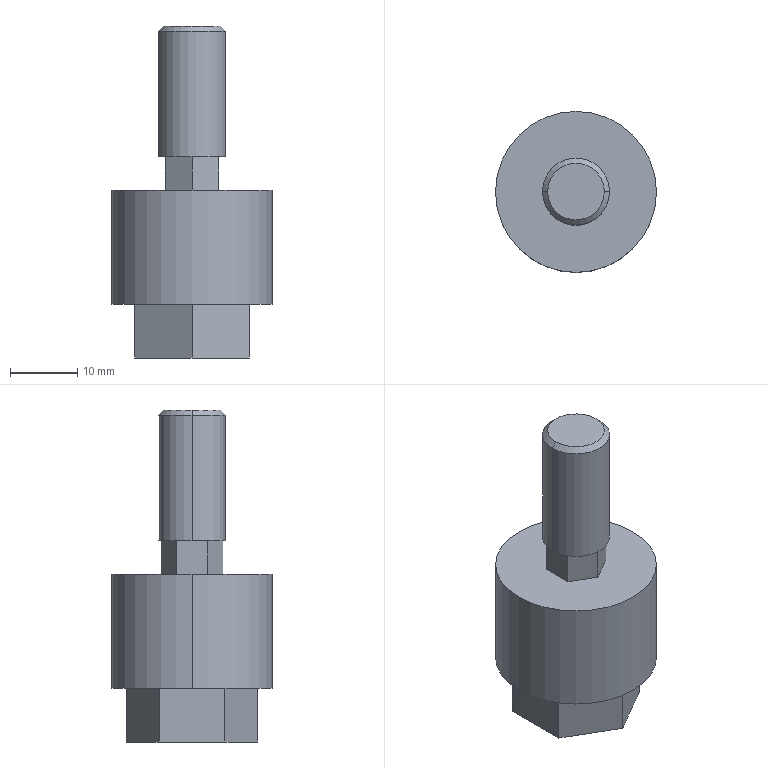Part | STEP file | JA30_10_125_JA30-10-125 | 1 solid | 28 faces | box 24 x 24 x 49.5 mm | volume 10958 mm3 | plane 18 | cylinder 6 | cone 4 | commonest cylinder face diameters 8.647 x2 10 x2 24 x2
STEP:
#1=CARTESIAN_POINT('',(-5.,0.,48.733));
#2=VERTEX_POINT('',#1);
#3=CARTESIAN_POINT('',(5.,0.,48.733));
#4=VERTEX_POINT('',#3);
#5=CARTESIAN_POINT('',(0.,0.,48.733));
#6=DIRECTION('',(0.,0.,-1.));
#7=DIRECTION('',(-1.,0.,0.));
#8=AXIS2_PLACEMENT_3D('',#5,#6,#7);
#9=CIRCLE('',#8,5.);
#10=EDGE_CURVE('',#2,#4,#9,.T.);
#11=ORIENTED_EDGE('',*,*,#10,.T.);
#12=CARTESIAN_POINT('',(5.,0.,30.));
#13=VERTEX_POINT('',#12);
#14=CARTESIAN_POINT('',(5.,0.,30.));
#15=DIRECTION('',(0.,0.,-1.));
#16=VECTOR('',#15,1000.);
#17=LINE('',#14,#16);
#18=EDGE_CURVE('',#4,#13,#17,.T.);
#19=ORIENTED_EDGE('',*,*,#18,.T.);
#20=CARTESIAN_POINT('',(-5.,0.,30.));
#21=VERTEX_POINT('',#20);
#22=CARTESIAN_POINT('',(0.,0.,30.));
#23=DIRECTION('',(0.,0.,-1.));
#24=DIRECTION('',(-1.,0.,0.));
#25=AXIS2_PLACEMENT_3D('',#22,#23,#24);
#26=CIRCLE('',#25,5.);
#27=EDGE_CURVE('',#21,#13,#26,.T.);
#28=ORIENTED_EDGE('',*,*,#27,.F.);
#29=CARTESIAN_POINT('',(-5.,0.,30.));
#30=DIRECTION('',(0.,0.,-1.));
#31=VECTOR('',#30,1000.);
#32=LINE('',#29,#31);
#33=EDGE_CURVE('',#2,#21,#32,.T.);
#34=ORIENTED_EDGE('',*,*,#33,.F.);
#35=EDGE_LOOP('',(#11,#19,#28,#34));
#36=FACE_OUTER_BOUND('',#35,.T.);
#37=CARTESIAN_POINT('',(0.,0.,30.));
#38=DIRECTION('',(0.,0.,-1.));
#39=DIRECTION('',(-1.,0.,0.));
#40=AXIS2_PLACEMENT_3D('',#37,#38,#39);
#41=CYLINDRICAL_SURFACE('',#40,5.);
#42=ADVANCED_FACE('',(#36),#41,.T.);
#43=CARTESIAN_POINT('',(-4.233,0.,49.5));
#44=VERTEX_POINT('',#43);
#45=CARTESIAN_POINT('',(4.233,0.,49.5));
#46=VERTEX_POINT('',#45);
#47=CARTESIAN_POINT('',(0.,0.,49.5));
#48=DIRECTION('',(0.,0.,-1.));
#49=DIRECTION('',(-1.,0.,0.));
#50=AXIS2_PLACEMENT_3D('',#47,#48,#49);
#51=CIRCLE('',#50,4.233);
#52=EDGE_CURVE('',#44,#46,#51,.T.);
#53=ORIENTED_EDGE('',*,*,#52,.T.);
#54=CARTESIAN_POINT('',(5.,0.,48.733));
#55=DIRECTION('',(0.7071,0.,-0.7071));
#56=VECTOR('',#55,1000.);
#57=LINE('',#54,#56);
#58=EDGE_CURVE('',#46,#4,#57,.T.);
#59=ORIENTED_EDGE('',*,*,#58,.T.);
#60=ORIENTED_EDGE('',*,*,#10,.F.);
#61=CARTESIAN_POINT('',(-5.,0.,48.733));
#62=DIRECTION('',(-0.7071,0.,-0.7071));
#63=VECTOR('',#62,1000.);
#64=LINE('',#61,#63);
#65=EDGE_CURVE('',#44,#2,#64,.T.);
#66=ORIENTED_EDGE('',*,*,#65,.F.);
#67=EDGE_LOOP('',(#53,#59,#60,#66));
#68=FACE_OUTER_BOUND('',#67,.T.);
#69=CARTESIAN_POINT('',(0.,0.,48.733));
#70=DIRECTION('',(0.,0.,-1.));
#71=DIRECTION('',(-1.,0.,0.));
#72=AXIS2_PLACEMENT_3D('',#69,#70,#71);
#73=CONICAL_SURFACE('',#72,5.,0.7854);
#74=ADVANCED_FACE('',(#68),#73,.T.);
#75=CARTESIAN_POINT('',(4.324,0.,0.6765));
#76=VERTEX_POINT('',#75);
#77=CARTESIAN_POINT('',(-4.324,0.,0.6765));
#78=VERTEX_POINT('',#77);
#79=CARTESIAN_POINT('',(0.,0.,0.6765));
#80=DIRECTION('',(0.,0.,-1.));
#81=DIRECTION('',(-1.,0.,0.));
#82=AXIS2_PLACEMENT_3D('',#79,#80,#81);
#83=CIRCLE('',#82,4.324);
#84=EDGE_CURVE('',#76,#78,#83,.T.);
#85=ORIENTED_EDGE('',*,*,#84,.F.);
#86=CARTESIAN_POINT('',(5.,0.,0.));
#87=VERTEX_POINT('',#86);
#88=CARTESIAN_POINT('',(4.324,0.,0.6765));
#89=DIRECTION('',(0.7071,0.,-0.7071));
#90=VECTOR('',#89,1000.);
#91=LINE('',#88,#90);
#92=EDGE_CURVE('',#76,#87,#91,.T.);
#93=ORIENTED_EDGE('',*,*,#92,.T.);
#94=CARTESIAN_POINT('',(-5.,0.,0.));
#95=VERTEX_POINT('',#94);
#96=CARTESIAN_POINT('',(0.,0.,0.));
#97=DIRECTION('',(0.,0.,-1.));
#98=DIRECTION('',(-1.,0.,0.));
#99=AXIS2_PLACEMENT_3D('',#96,#97,#98);
#100=CIRCLE('',#99,5.);
#101=EDGE_CURVE('',#87,#95,#100,.T.);
#102=ORIENTED_EDGE('',*,*,#101,.T.);
#103=CARTESIAN_POINT('',(-4.324,0.,0.6765));
#104=DIRECTION('',(-0.7071,0.,-0.7071));
#105=VECTOR('',#104,1000.);
#106=LINE('',#103,#105);
#107=EDGE_CURVE('',#78,#95,#106,.T.);
#108=ORIENTED_EDGE('',*,*,#107,.F.);
#109=EDGE_LOOP('',(#85,#93,#102,#108));
#110=FACE_OUTER_BOUND('',#109,.T.);
#111=CARTESIAN_POINT('',(0.,0.,0.6765));
#112=DIRECTION('',(0.,0.,-1.));
#113=DIRECTION('',(-1.,0.,0.));
#114=AXIS2_PLACEMENT_3D('',#111,#112,#113);
#115=CONICAL_SURFACE('',#114,4.324,0.7854);
#116=ADVANCED_FACE('',(#110),#115,.F.);
#117=CARTESIAN_POINT('',(4.324,0.,9.));
#118=VERTEX_POINT('',#117);
#119=CARTESIAN_POINT('',(-4.324,0.,9.));
#120=VERTEX_POINT('',#119);
#121=CARTESIAN_POINT('',(0.,0.,9.));
#122=DIRECTION('',(0.,0.,-1.));
#123=DIRECTION('',(-1.,0.,0.));
#124=AXIS2_PLACEMENT_3D('',#121,#122,#123);
#125=CIRCLE('',#124,4.324);
#126=EDGE_CURVE('',#118,#120,#125,.T.);
#127=ORIENTED_EDGE('',*,*,#126,.F.);
#128=CARTESIAN_POINT('',(4.324,0.,0.));
#129=DIRECTION('',(0.,0.,-1.));
#130=VECTOR('',#129,1000.);
#131=LINE('',#128,#130);
#132=EDGE_CURVE('',#118,#76,#131,.T.);
#133=ORIENTED_EDGE('',*,*,#132,.T.);
#134=ORIENTED_EDGE('',*,*,#84,.T.);
#135=CARTESIAN_POINT('',(-4.324,0.,0.));
#136=DIRECTION('',(0.,0.,-1.));
#137=VECTOR('',#136,1000.);
#138=LINE('',#135,#137);
#139=EDGE_CURVE('',#120,#78,#138,.T.);
#140=ORIENTED_EDGE('',*,*,#139,.F.);
#141=EDGE_LOOP('',(#127,#133,#134,#140));
#142=FACE_OUTER_BOUND('',#141,.T.);
#143=CARTESIAN_POINT('',(0.,0.,0.));
#144=DIRECTION('',(0.,0.,-1.));
#145=DIRECTION('',(-1.,0.,0.));
#146=AXIS2_PLACEMENT_3D('',#143,#144,#145);
#147=CYLINDRICAL_SURFACE('',#146,4.324);
#148=ADVANCED_FACE('',(#142),#147,.F.);
#149=CARTESIAN_POINT('',(-12.,0.,25.));
#150=VERTEX_POINT('',#149);
#151=CARTESIAN_POINT('',(12.,0.,25.));
#152=VERTEX_POINT('',#151);
#153=CARTESIAN_POINT('',(0.,0.,25.));
#154=DIRECTION('',(0.,0.,-1.));
#155=DIRECTION('',(-1.,0.,0.));
#156=AXIS2_PLACEMENT_3D('',#153,#154,#155);
#157=CIRCLE('',#156,12.);
#158=EDGE_CURVE('',#150,#152,#157,.T.);
#159=ORIENTED_EDGE('',*,*,#158,.T.);
#160=CARTESIAN_POINT('',(12.,0.,8.));
#161=VERTEX_POINT('',#160);
#162=CARTESIAN_POINT('',(12.,0.,0.));
#163=DIRECTION('',(0.,0.,-1.));
#164=VECTOR('',#163,1000.);
#165=LINE('',#162,#164);
#166=EDGE_CURVE('',#152,#161,#165,.T.);
#167=ORIENTED_EDGE('',*,*,#166,.T.);
#168=CARTESIAN_POINT('',(-12.,0.,8.));
#169=VERTEX_POINT('',#168);
#170=CARTESIAN_POINT('',(0.,0.,8.));
#171=DIRECTION('',(0.,0.,-1.));
#172=DIRECTION('',(-1.,0.,0.));
#173=AXIS2_PLACEMENT_3D('',#170,#171,#172);
#174=CIRCLE('',#173,12.);
#175=EDGE_CURVE('',#169,#161,#174,.T.);
#176=ORIENTED_EDGE('',*,*,#175,.F.);
#177=CARTESIAN_POINT('',(-12.,0.,0.));
#178=DIRECTION('',(0.,0.,-1.));
#179=VECTOR('',#178,1000.);
#180=LINE('',#177,#179);
#181=EDGE_CURVE('',#150,#169,#180,.T.);
#182=ORIENTED_EDGE('',*,*,#181,.F.);
#183=EDGE_LOOP('',(#159,#167,#176,#182));
#184=FACE_OUTER_BOUND('',#183,.T.);
#185=CARTESIAN_POINT('',(0.,0.,0.));
#186=DIRECTION('',(0.,0.,-1.));
#187=DIRECTION('',(-1.,0.,0.));
#188=AXIS2_PLACEMENT_3D('',#185,#186,#187);
#189=CYLINDRICAL_SURFACE('',#188,12.);
#190=ADVANCED_FACE('',(#184),#189,.T.);
#191=CARTESIAN_POINT('',(0.,4.619,30.));
#192=VERTEX_POINT('',#191);
#193=CARTESIAN_POINT('',(-4.,2.309,30.));
#194=VERTEX_POINT('',#193);
#195=CARTESIAN_POINT('',(0.,4.619,30.));
#196=DIRECTION('',(-0.866,-0.5,0.));
#197=VECTOR('',#196,1000.);
#198=LINE('',#195,#197);
#199=EDGE_CURVE('',#192,#194,#198,.T.);
#200=ORIENTED_EDGE('',*,*,#199,.F.);
#201=CARTESIAN_POINT('',(0.,4.619,25.));
#202=VERTEX_POINT('',#201);
#203=CARTESIAN_POINT('',(0.,4.619,25.));
#204=DIRECTION('',(0.,0.,1.));
#205=VECTOR('',#204,1000.);
#206=LINE('',#203,#205);
#207=EDGE_CURVE('',#202,#192,#206,.T.);
#208=ORIENTED_EDGE('',*,*,#207,.F.);
#209=CARTESIAN_POINT('',(-4.,2.309,25.));
#210=VERTEX_POINT('',#209);
#211=CARTESIAN_POINT('',(0.,4.619,25.));
#212=DIRECTION('',(-0.866,-0.5,0.));
#213=VECTOR('',#212,1000.);
#214=LINE('',#211,#213);
#215=EDGE_CURVE('',#202,#210,#214,.T.);
#216=ORIENTED_EDGE('',*,*,#215,.T.);
#217=CARTESIAN_POINT('',(-4.,2.309,25.));
#218=DIRECTION('',(0.,0.,1.));
#219=VECTOR('',#218,1000.);
#220=LINE('',#217,#219);
#221=EDGE_CURVE('',#210,#194,#220,.T.);
#222=ORIENTED_EDGE('',*,*,#221,.T.);
#223=EDGE_LOOP('',(#200,#208,#216,#222));
#224=FACE_OUTER_BOUND('',#223,.T.);
#225=CARTESIAN_POINT('',(0.,4.619,25.));
#226=DIRECTION('',(-0.5,0.866,0.));
#227=DIRECTION('',(-0.866,-0.5,0.));
#228=AXIS2_PLACEMENT_3D('',#225,#226,#227);
#229=PLANE('',#228);
#230=ADVANCED_FACE('',(#224),#229,.T.);
#231=CARTESIAN_POINT('',(4.,2.309,30.));
#232=VERTEX_POINT('',#231);
#233=CARTESIAN_POINT('',(4.,2.309,30.));
#234=DIRECTION('',(-0.866,0.5,0.));
#235=VECTOR('',#234,1000.);
#236=LINE('',#233,#235);
#237=EDGE_CURVE('',#232,#192,#236,.T.);
#238=ORIENTED_EDGE('',*,*,#237,.F.);
#239=CARTESIAN_POINT('',(4.,2.309,25.));
#240=VERTEX_POINT('',#239);
#241=CARTESIAN_POINT('',(4.,2.309,25.));
#242=DIRECTION('',(0.,0.,1.));
#243=VECTOR('',#242,1000.);
#244=LINE('',#241,#243);
#245=EDGE_CURVE('',#240,#232,#244,.T.);
#246=ORIENTED_EDGE('',*,*,#245,.F.);
#247=CARTESIAN_POINT('',(4.,2.309,25.));
#248=DIRECTION('',(-0.866,0.5,0.));
#249=VECTOR('',#248,1000.);
#250=LINE('',#247,#249);
#251=EDGE_CURVE('',#240,#202,#250,.T.);
#252=ORIENTED_EDGE('',*,*,#251,.T.);
#253=ORIENTED_EDGE('',*,*,#207,.T.);
#254=EDGE_LOOP('',(#238,#246,#252,#253));
#255=FACE_OUTER_BOUND('',#254,.T.);
#256=CARTESIAN_POINT('',(4.,2.309,25.));
#257=DIRECTION('',(0.5,0.866,0.));
#258=DIRECTION('',(-0.866,0.5,0.));
#259=AXIS2_PLACEMENT_3D('',#256,#257,#258);
#260=PLANE('',#259);
#261=ADVANCED_FACE('',(#255),#260,.T.);
#262=CARTESIAN_POINT('',(4.,-2.309,30.));
#263=VERTEX_POINT('',#262);
#264=CARTESIAN_POINT('',(4.,-2.309,30.));
#265=DIRECTION('',(0.,1.,0.));
#266=VECTOR('',#265,1000.);
#267=LINE('',#264,#266);
#268=EDGE_CURVE('',#263,#232,#267,.T.);
#269=ORIENTED_EDGE('',*,*,#268,.F.);
#270=CARTESIAN_POINT('',(4.,-2.309,25.));
#271=VERTEX_POINT('',#270);
#272=CARTESIAN_POINT('',(4.,-2.309,25.));
#273=DIRECTION('',(0.,0.,1.));
#274=VECTOR('',#273,1000.);
#275=LINE('',#272,#274);
#276=EDGE_CURVE('',#271,#263,#275,.T.);
#277=ORIENTED_EDGE('',*,*,#276,.F.);
#278=CARTESIAN_POINT('',(4.,-2.309,25.));
#279=DIRECTION('',(0.,1.,0.));
#280=VECTOR('',#279,1000.);
#281=LINE('',#278,#280);
#282=EDGE_CURVE('',#271,#240,#281,.T.);
#283=ORIENTED_EDGE('',*,*,#282,.T.);
#284=ORIENTED_EDGE('',*,*,#245,.T.);
#285=EDGE_LOOP('',(#269,#277,#283,#284));
#286=FACE_OUTER_BOUND('',#285,.T.);
#287=CARTESIAN_POINT('',(4.,-2.309,25.));
#288=DIRECTION('',(1.,0.,0.));
#289=DIRECTION('',(0.,0.,-1.));
#290=AXIS2_PLACEMENT_3D('',#287,#288,#289);
#291=PLANE('',#290);
#292=ADVANCED_FACE('',(#286),#291,.T.);
#293=CARTESIAN_POINT('',(0.,-4.619,30.));
#294=VERTEX_POINT('',#293);
#295=CARTESIAN_POINT('',(0.,-4.619,30.));
#296=DIRECTION('',(0.866,0.5,0.));
#297=VECTOR('',#296,1000.);
#298=LINE('',#295,#297);
#299=EDGE_CURVE('',#294,#263,#298,.T.);
#300=ORIENTED_EDGE('',*,*,#299,.F.);
#301=CARTESIAN_POINT('',(0.,-4.619,25.));
#302=VERTEX_POINT('',#301);
#303=CARTESIAN_POINT('',(0.,-4.619,25.));
#304=DIRECTION('',(0.,0.,1.));
#305=VECTOR('',#304,1000.);
#306=LINE('',#303,#305);
#307=EDGE_CURVE('',#302,#294,#306,.T.);
#308=ORIENTED_EDGE('',*,*,#307,.F.);
#309=CARTESIAN_POINT('',(0.,-4.619,25.));
#310=DIRECTION('',(0.866,0.5,0.));
#311=VECTOR('',#310,1000.);
#312=LINE('',#309,#311);
#313=EDGE_CURVE('',#302,#271,#312,.T.);
#314=ORIENTED_EDGE('',*,*,#313,.T.);
#315=ORIENTED_EDGE('',*,*,#276,.T.);
#316=EDGE_LOOP('',(#300,#308,#314,#315));
#317=FACE_OUTER_BOUND('',#316,.T.);
#318=CARTESIAN_POINT('',(0.,-4.619,25.));
#319=DIRECTION('',(0.5,-0.866,0.));
#320=DIRECTION('',(0.866,0.5,0.));
#321=AXIS2_PLACEMENT_3D('',#318,#319,#320);
#322=PLANE('',#321);
#323=ADVANCED_FACE('',(#317),#322,.T.);
#324=CARTESIAN_POINT('',(-4.,-2.309,30.));
#325=VERTEX_POINT('',#324);
#326=CARTESIAN_POINT('',(-4.,-2.309,30.));
#327=DIRECTION('',(0.866,-0.5,0.));
#328=VECTOR('',#327,1000.);
#329=LINE('',#326,#328);
#330=EDGE_CURVE('',#325,#294,#329,.T.);
#331=ORIENTED_EDGE('',*,*,#330,.F.);
#332=CARTESIAN_POINT('',(-4.,-2.309,25.));
#333=VERTEX_POINT('',#332);
#334=CARTESIAN_POINT('',(-4.,-2.309,25.));
#335=DIRECTION('',(0.,0.,1.));
#336=VECTOR('',#335,1000.);
#337=LINE('',#334,#336);
#338=EDGE_CURVE('',#333,#325,#337,.T.);
#339=ORIENTED_EDGE('',*,*,#338,.F.);
#340=CARTESIAN_POINT('',(-4.,-2.309,25.));
#341=DIRECTION('',(0.866,-0.5,0.));
#342=VECTOR('',#341,1000.);
#343=LINE('',#340,#342);
#344=EDGE_CURVE('',#333,#302,#343,.T.);
#345=ORIENTED_EDGE('',*,*,#344,.T.);
#346=ORIENTED_EDGE('',*,*,#307,.T.);
#347=EDGE_LOOP('',(#331,#339,#345,#346));
#348=FACE_OUTER_BOUND('',#347,.T.);
#349=CARTESIAN_POINT('',(-4.,-2.309,25.));
#350=DIRECTION('',(-0.5,-0.866,0.));
#351=DIRECTION('',(0.866,-0.5,0.));
#352=AXIS2_PLACEMENT_3D('',#349,#350,#351);
#353=PLANE('',#352);
#354=ADVANCED_FACE('',(#348),#353,.T.);
#355=CARTESIAN_POINT('',(-4.,2.309,30.));
#356=DIRECTION('',(0.,-1.,0.));
#357=VECTOR('',#356,1000.);
#358=LINE('',#355,#357);
#359=EDGE_CURVE('',#194,#325,#358,.T.);
#360=ORIENTED_EDGE('',*,*,#359,.F.);
#361=ORIENTED_EDGE('',*,*,#221,.F.);
#362=CARTESIAN_POINT('',(-4.,2.309,25.));
#363=DIRECTION('',(0.,-1.,0.));
#364=VECTOR('',#363,1000.);
#365=LINE('',#362,#364);
#366=EDGE_CURVE('',#210,#333,#365,.T.);
#367=ORIENTED_EDGE('',*,*,#366,.T.);
#368=ORIENTED_EDGE('',*,*,#338,.T.);
#369=EDGE_LOOP('',(#360,#361,#367,#368));
#370=FACE_OUTER_BOUND('',#369,.T.);
#371=CARTESIAN_POINT('',(-4.,2.309,25.));
#372=DIRECTION('',(-1.,0.,0.));
#373=DIRECTION('',(0.,0.,1.));
#374=AXIS2_PLACEMENT_3D('',#371,#372,#373);
#375=PLANE('',#374);
#376=ADVANCED_FACE('',(#370),#375,.T.);
#377=ORIENTED_EDGE('',*,*,#366,.F.);
#378=ORIENTED_EDGE('',*,*,#215,.F.);
#379=ORIENTED_EDGE('',*,*,#251,.F.);
#380=ORIENTED_EDGE('',*,*,#282,.F.);
#381=ORIENTED_EDGE('',*,*,#313,.F.);
#382=ORIENTED_EDGE('',*,*,#344,.F.);
#383=EDGE_LOOP('',(#377,#378,#379,#380,#381,#382));
#384=FACE_BOUND('',#383,.T.);
#385=ORIENTED_EDGE('',*,*,#158,.F.);
#386=CARTESIAN_POINT('',(0.,0.,25.));
#387=DIRECTION('',(0.,0.,-1.));
#388=DIRECTION('',(-1.,0.,0.));
#389=AXIS2_PLACEMENT_3D('',#386,#387,#388);
#390=CIRCLE('',#389,12.);
#391=EDGE_CURVE('',#152,#150,#390,.T.);
#392=ORIENTED_EDGE('',*,*,#391,.F.);
#393=EDGE_LOOP('',(#385,#392));
#394=FACE_OUTER_BOUND('',#393,.T.);
#395=CARTESIAN_POINT('',(0.,0.,25.));
#396=DIRECTION('',(0.,0.,1.));
#397=DIRECTION('',(1.,0.,0.));
#398=AXIS2_PLACEMENT_3D('',#395,#396,#397);
#399=PLANE('',#398);
#400=ADVANCED_FACE('',(#384,#394),#399,.T.);
#401=ORIENTED_EDGE('',*,*,#166,.F.);
#402=ORIENTED_EDGE('',*,*,#391,.T.);
#403=ORIENTED_EDGE('',*,*,#181,.T.);
#404=CARTESIAN_POINT('',(0.,0.,8.));
#405=DIRECTION('',(0.,0.,-1.));
#406=DIRECTION('',(-1.,0.,0.));
#407=AXIS2_PLACEMENT_3D('',#404,#405,#406);
#408=CIRCLE('',#407,12.);
#409=EDGE_CURVE('',#161,#169,#408,.T.);
#410=ORIENTED_EDGE('',*,*,#409,.F.);
#411=EDGE_LOOP('',(#401,#402,#403,#410));
#412=FACE_OUTER_BOUND('',#411,.T.);
#413=CARTESIAN_POINT('',(0.,0.,0.));
#414=DIRECTION('',(0.,0.,-1.));
#415=DIRECTION('',(-1.,0.,0.));
#416=AXIS2_PLACEMENT_3D('',#413,#414,#415);
#417=CYLINDRICAL_SURFACE('',#416,12.);
#418=ADVANCED_FACE('',(#412),#417,.T.);
#419=ORIENTED_EDGE('',*,*,#175,.T.);
#420=ORIENTED_EDGE('',*,*,#409,.T.);
#421=EDGE_LOOP('',(#419,#420));
#422=FACE_OUTER_BOUND('',#421,.T.);
#423=CARTESIAN_POINT('',(-8.5,4.907,8.));
#424=VERTEX_POINT('',#423);
#425=CARTESIAN_POINT('',(-8.5,-4.907,8.));
#426=VERTEX_POINT('',#425);
#427=CARTESIAN_POINT('',(-8.5,4.907,8.));
#428=DIRECTION('',(0.,-1.,0.));
#429=VECTOR('',#428,1000.);
#430=LINE('',#427,#429);
#431=EDGE_CURVE('',#424,#426,#430,.T.);
#432=ORIENTED_EDGE('',*,*,#431,.T.);
#433=CARTESIAN_POINT('',(0.,-9.815,8.));
#434=VERTEX_POINT('',#433);
#435=CARTESIAN_POINT('',(-8.5,-4.907,8.));
#436=DIRECTION('',(0.866,-0.5,0.));
#437=VECTOR('',#436,1000.);
#438=LINE('',#435,#437);
#439=EDGE_CURVE('',#426,#434,#438,.T.);
#440=ORIENTED_EDGE('',*,*,#439,.T.);
#441=CARTESIAN_POINT('',(8.5,-4.907,8.));
#442=VERTEX_POINT('',#441);
#443=CARTESIAN_POINT('',(0.,-9.815,8.));
#444=DIRECTION('',(0.866,0.5,0.));
#445=VECTOR('',#444,1000.);
#446=LINE('',#443,#445);
#447=EDGE_CURVE('',#434,#442,#446,.T.);
#448=ORIENTED_EDGE('',*,*,#447,.T.);
#449=CARTESIAN_POINT('',(8.5,4.907,8.));
#450=VERTEX_POINT('',#449);
#451=CARTESIAN_POINT('',(8.5,-4.907,8.));
#452=DIRECTION('',(0.,1.,0.));
#453=VECTOR('',#452,1000.);
#454=LINE('',#451,#453);
#455=EDGE_CURVE('',#442,#450,#454,.T.);
#456=ORIENTED_EDGE('',*,*,#455,.T.);
#457=CARTESIAN_POINT('',(0.,9.815,8.));
#458=VERTEX_POINT('',#457);
#459=CARTESIAN_POINT('',(8.5,4.907,8.));
#460=DIRECTION('',(-0.866,0.5,0.));
#461=VECTOR('',#460,1000.);
#462=LINE('',#459,#461);
#463=EDGE_CURVE('',#450,#458,#462,.T.);
#464=ORIENTED_EDGE('',*,*,#463,.T.);
#465=CARTESIAN_POINT('',(0.,9.815,8.));
#466=DIRECTION('',(-0.866,-0.5,0.));
#467=VECTOR('',#466,1000.);
#468=LINE('',#465,#467);
#469=EDGE_CURVE('',#458,#424,#468,.T.);
#470=ORIENTED_EDGE('',*,*,#469,.T.);
#471=EDGE_LOOP('',(#432,#440,#448,#456,#464,#470));
#472=FACE_BOUND('',#471,.T.);
#473=CARTESIAN_POINT('',(0.,12.,8.));
#474=DIRECTION('',(0.,0.,-1.));
#475=DIRECTION('',(-1.,0.,0.));
#476=AXIS2_PLACEMENT_3D('',#473,#474,#475);
#477=PLANE('',#476);
#478=ADVANCED_FACE('',(#422,#472),#477,.T.);
#479=CARTESIAN_POINT('',(0.,9.815,0.));
#480=VERTEX_POINT('',#479);
#481=CARTESIAN_POINT('',(-8.5,4.907,0.));
#482=VERTEX_POINT('',#481);
#483=CARTESIAN_POINT('',(0.,9.815,0.));
#484=DIRECTION('',(-0.866,-0.5,0.));
#485=VECTOR('',#484,1000.);
#486=LINE('',#483,#485);
#487=EDGE_CURVE('',#480,#482,#486,.T.);
#488=ORIENTED_EDGE('',*,*,#487,.T.);
#489=CARTESIAN_POINT('',(-8.5,4.907,8.));
#490=DIRECTION('',(0.,0.,-1.));
#491=VECTOR('',#490,1000.);
#492=LINE('',#489,#491);
#493=EDGE_CURVE('',#424,#482,#492,.T.);
#494=ORIENTED_EDGE('',*,*,#493,.F.);
#495=ORIENTED_EDGE('',*,*,#469,.F.);
#496=CARTESIAN_POINT('',(0.,9.815,8.));
#497=DIRECTION('',(0.,0.,-1.));
#498=VECTOR('',#497,1000.);
#499=LINE('',#496,#498);
#500=EDGE_CURVE('',#458,#480,#499,.T.);
#501=ORIENTED_EDGE('',*,*,#500,.T.);
#502=EDGE_LOOP('',(#488,#494,#495,#501));
#503=FACE_OUTER_BOUND('',#502,.T.);
#504=CARTESIAN_POINT('',(0.,9.815,8.));
#505=DIRECTION('',(0.5,-0.866,0.));
#506=DIRECTION('',(0.866,0.5,0.));
#507=AXIS2_PLACEMENT_3D('',#504,#505,#506);
#508=PLANE('',#507);
#509=ADVANCED_FACE('',(#503),#508,.F.);
#510=CARTESIAN_POINT('',(-8.5,-4.907,0.));
#511=VERTEX_POINT('',#510);
#512=CARTESIAN_POINT('',(-8.5,4.907,0.));
#513=DIRECTION('',(0.,-1.,0.));
#514=VECTOR('',#513,1000.);
#515=LINE('',#512,#514);
#516=EDGE_CURVE('',#482,#511,#515,.T.);
#517=ORIENTED_EDGE('',*,*,#516,.T.);
#518=CARTESIAN_POINT('',(-8.5,-4.907,8.));
#519=DIRECTION('',(0.,0.,-1.));
#520=VECTOR('',#519,1000.);
#521=LINE('',#518,#520);
#522=EDGE_CURVE('',#426,#511,#521,.T.);
#523=ORIENTED_EDGE('',*,*,#522,.F.);
#524=ORIENTED_EDGE('',*,*,#431,.F.);
#525=ORIENTED_EDGE('',*,*,#493,.T.);
#526=EDGE_LOOP('',(#517,#523,#524,#525));
#527=FACE_OUTER_BOUND('',#526,.T.);
#528=CARTESIAN_POINT('',(-8.5,4.907,8.));
#529=DIRECTION('',(1.,0.,0.));
#530=DIRECTION('',(0.,0.,-1.));
#531=AXIS2_PLACEMENT_3D('',#528,#529,#530);
#532=PLANE('',#531);
#533=ADVANCED_FACE('',(#527),#532,.F.);
#534=CARTESIAN_POINT('',(0.,-9.815,0.));
#535=VERTEX_POINT('',#534);
#536=CARTESIAN_POINT('',(-8.5,-4.907,0.));
#537=DIRECTION('',(0.866,-0.5,0.));
#538=VECTOR('',#537,1000.);
#539=LINE('',#536,#538);
#540=EDGE_CURVE('',#511,#535,#539,.T.);
#541=ORIENTED_EDGE('',*,*,#540,.T.);
#542=CARTESIAN_POINT('',(0.,-9.815,8.));
#543=DIRECTION('',(0.,0.,-1.));
#544=VECTOR('',#543,1000.);
#545=LINE('',#542,#544);
#546=EDGE_CURVE('',#434,#535,#545,.T.);
#547=ORIENTED_EDGE('',*,*,#546,.F.);
#548=ORIENTED_EDGE('',*,*,#439,.F.);
#549=ORIENTED_EDGE('',*,*,#522,.T.);
#550=EDGE_LOOP('',(#541,#547,#548,#549));
#551=FACE_OUTER_BOUND('',#550,.T.);
#552=CARTESIAN_POINT('',(-8.5,-4.907,8.));
#553=DIRECTION('',(0.5,0.866,0.));
#554=DIRECTION('',(-0.866,0.5,0.));
#555=AXIS2_PLACEMENT_3D('',#552,#553,#554);
#556=PLANE('',#555);
#557=ADVANCED_FACE('',(#551),#556,.F.);
#558=CARTESIAN_POINT('',(8.5,-4.907,0.));
#559=VERTEX_POINT('',#558);
#560=CARTESIAN_POINT('',(0.,-9.815,0.));
#561=DIRECTION('',(0.866,0.5,0.));
#562=VECTOR('',#561,1000.);
#563=LINE('',#560,#562);
#564=EDGE_CURVE('',#535,#559,#563,.T.);
#565=ORIENTED_EDGE('',*,*,#564,.T.);
#566=CARTESIAN_POINT('',(8.5,-4.907,8.));
#567=DIRECTION('',(0.,0.,-1.));
#568=VECTOR('',#567,1000.);
#569=LINE('',#566,#568);
#570=EDGE_CURVE('',#442,#559,#569,.T.);
#571=ORIENTED_EDGE('',*,*,#570,.F.);
#572=ORIENTED_EDGE('',*,*,#447,.F.);
#573=ORIENTED_EDGE('',*,*,#546,.T.);
#574=EDGE_LOOP('',(#565,#571,#572,#573));
#575=FACE_OUTER_BOUND('',#574,.T.);
#576=CARTESIAN_POINT('',(0.,-9.815,8.));
#577=DIRECTION('',(-0.5,0.866,0.));
#578=DIRECTION('',(-0.866,-0.5,0.));
#579=AXIS2_PLACEMENT_3D('',#576,#577,#578);
#580=PLANE('',#579);
#581=ADVANCED_FACE('',(#575),#580,.F.);
#582=CARTESIAN_POINT('',(8.5,4.907,0.));
#583=VERTEX_POINT('',#582);
#584=CARTESIAN_POINT('',(8.5,-4.907,0.));
#585=DIRECTION('',(0.,1.,0.));
#586=VECTOR('',#585,1000.);
#587=LINE('',#584,#586);
#588=EDGE_CURVE('',#559,#583,#587,.T.);
#589=ORIENTED_EDGE('',*,*,#588,.T.);
#590=CARTESIAN_POINT('',(8.5,4.907,8.));
#591=DIRECTION('',(0.,0.,-1.));
#592=VECTOR('',#591,1000.);
#593=LINE('',#590,#592);
#594=EDGE_CURVE('',#450,#583,#593,.T.);
#595=ORIENTED_EDGE('',*,*,#594,.F.);
#596=ORIENTED_EDGE('',*,*,#455,.F.);
#597=ORIENTED_EDGE('',*,*,#570,.T.);
#598=EDGE_LOOP('',(#589,#595,#596,#597));
#599=FACE_OUTER_BOUND('',#598,.T.);
#600=CARTESIAN_POINT('',(8.5,-4.907,8.));
#601=DIRECTION('',(-1.,0.,0.));
#602=DIRECTION('',(0.,0.,1.));
#603=AXIS2_PLACEMENT_3D('',#600,#601,#602);
#604=PLANE('',#603);
#605=ADVANCED_FACE('',(#599),#604,.F.);
#606=CARTESIAN_POINT('',(8.5,4.907,0.));
#607=DIRECTION('',(-0.866,0.5,0.));
#608=VECTOR('',#607,1000.);
#609=LINE('',#606,#608);
#610=EDGE_CURVE('',#583,#480,#609,.T.);
#611=ORIENTED_EDGE('',*,*,#610,.T.);
#612=ORIENTED_EDGE('',*,*,#500,.F.);
#613=ORIENTED_EDGE('',*,*,#463,.F.);
#614=ORIENTED_EDGE('',*,*,#594,.T.);
#615=EDGE_LOOP('',(#611,#612,#613,#614));
#616=FACE_OUTER_BOUND('',#615,.T.);
#617=CARTESIAN_POINT('',(8.5,4.907,8.));
#618=DIRECTION('',(-0.5,-0.866,0.));
#619=DIRECTION('',(0.866,-0.5,0.));
#620=AXIS2_PLACEMENT_3D('',#617,#618,#619);
#621=PLANE('',#620);
#622=ADVANCED_FACE('',(#616),#621,.F.);
#623=CARTESIAN_POINT('',(0.,0.,9.));
#624=DIRECTION('',(0.,0.,-1.));
#625=DIRECTION('',(-1.,0.,0.));
#626=AXIS2_PLACEMENT_3D('',#623,#624,#625);
#627=CIRCLE('',#626,4.324);
#628=EDGE_CURVE('',#120,#118,#627,.T.);
#629=ORIENTED_EDGE('',*,*,#628,.T.);
#630=ORIENTED_EDGE('',*,*,#126,.T.);
#631=EDGE_LOOP('',(#629,#630));
#632=FACE_OUTER_BOUND('',#631,.T.);
#633=CARTESIAN_POINT('',(0.,4.324,9.));
#634=DIRECTION('',(0.,0.,-1.));
#635=DIRECTION('',(-1.,0.,0.));
#636=AXIS2_PLACEMENT_3D('',#633,#634,#635);
#637=PLANE('',#636);
#638=ADVANCED_FACE('',(#632),#637,.T.);
#639=ORIENTED_EDGE('',*,*,#132,.F.);
#640=ORIENTED_EDGE('',*,*,#628,.F.);
#641=ORIENTED_EDGE('',*,*,#139,.T.);
#642=CARTESIAN_POINT('',(0.,0.,0.6765));
#643=DIRECTION('',(0.,0.,-1.));
#644=DIRECTION('',(-1.,0.,0.));
#645=AXIS2_PLACEMENT_3D('',#642,#643,#644);
#646=CIRCLE('',#645,4.324);
#647=EDGE_CURVE('',#78,#76,#646,.T.);
#648=ORIENTED_EDGE('',*,*,#647,.T.);
#649=EDGE_LOOP('',(#639,#640,#641,#648));
#650=FACE_OUTER_BOUND('',#649,.T.);
#651=CARTESIAN_POINT('',(0.,0.,0.));
#652=DIRECTION('',(0.,0.,-1.));
#653=DIRECTION('',(-1.,0.,0.));
#654=AXIS2_PLACEMENT_3D('',#651,#652,#653);
#655=CYLINDRICAL_SURFACE('',#654,4.324);
#656=ADVANCED_FACE('',(#650),#655,.F.);
#657=ORIENTED_EDGE('',*,*,#92,.F.);
#658=ORIENTED_EDGE('',*,*,#647,.F.);
#659=ORIENTED_EDGE('',*,*,#107,.T.);
#660=CARTESIAN_POINT('',(0.,0.,0.));
#661=DIRECTION('',(0.,0.,-1.));
#662=DIRECTION('',(-1.,0.,0.));
#663=AXIS2_PLACEMENT_3D('',#660,#661,#662);
#664=CIRCLE('',#663,5.);
#665=EDGE_CURVE('',#95,#87,#664,.T.);
#666=ORIENTED_EDGE('',*,*,#665,.T.);
#667=EDGE_LOOP('',(#657,#658,#659,#666));
#668=FACE_OUTER_BOUND('',#667,.T.);
#669=CARTESIAN_POINT('',(0.,0.,0.6765));
#670=DIRECTION('',(0.,0.,-1.));
#671=DIRECTION('',(-1.,0.,0.));
#672=AXIS2_PLACEMENT_3D('',#669,#670,#671);
#673=CONICAL_SURFACE('',#672,4.324,0.7854);
#674=ADVANCED_FACE('',(#668),#673,.F.);
#675=ORIENTED_EDGE('',*,*,#487,.F.);
#676=ORIENTED_EDGE('',*,*,#610,.F.);
#677=ORIENTED_EDGE('',*,*,#588,.F.);
#678=ORIENTED_EDGE('',*,*,#564,.F.);
#679=ORIENTED_EDGE('',*,*,#540,.F.);
#680=ORIENTED_EDGE('',*,*,#516,.F.);
#681=EDGE_LOOP('',(#675,#676,#677,#678,#679,#680));
#682=FACE_OUTER_BOUND('',#681,.T.);
#683=ORIENTED_EDGE('',*,*,#665,.F.);
#684=ORIENTED_EDGE('',*,*,#101,.F.);
#685=EDGE_LOOP('',(#683,#684));
#686=FACE_BOUND('',#685,.T.);
#687=CARTESIAN_POINT('',(0.,10.2,0.));
#688=DIRECTION('',(0.,0.,-1.));
#689=DIRECTION('',(-1.,0.,0.));
#690=AXIS2_PLACEMENT_3D('',#687,#688,#689);
#691=PLANE('',#690);
#692=ADVANCED_FACE('',(#682,#686),#691,.T.);
#693=ORIENTED_EDGE('',*,*,#52,.F.);
#694=CARTESIAN_POINT('',(0.,0.,49.5));
#695=DIRECTION('',(0.,0.,-1.));
#696=DIRECTION('',(-1.,0.,0.));
#697=AXIS2_PLACEMENT_3D('',#694,#695,#696);
#698=CIRCLE('',#697,4.233);
#699=EDGE_CURVE('',#46,#44,#698,.T.);
#700=ORIENTED_EDGE('',*,*,#699,.F.);
#701=EDGE_LOOP('',(#693,#700));
#702=FACE_OUTER_BOUND('',#701,.T.);
#703=CARTESIAN_POINT('',(0.,0.,49.5));
#704=DIRECTION('',(0.,0.,1.));
#705=DIRECTION('',(1.,0.,0.));
#706=AXIS2_PLACEMENT_3D('',#703,#704,#705);
#707=PLANE('',#706);
#708=ADVANCED_FACE('',(#702),#707,.T.);
#709=ORIENTED_EDGE('',*,*,#58,.F.);
#710=ORIENTED_EDGE('',*,*,#699,.T.);
#711=ORIENTED_EDGE('',*,*,#65,.T.);
#712=CARTESIAN_POINT('',(0.,0.,48.733));
#713=DIRECTION('',(0.,0.,-1.));
#714=DIRECTION('',(-1.,0.,0.));
#715=AXIS2_PLACEMENT_3D('',#712,#713,#714);
#716=CIRCLE('',#715,5.);
#717=EDGE_CURVE('',#4,#2,#716,.T.);
#718=ORIENTED_EDGE('',*,*,#717,.F.);
#719=EDGE_LOOP('',(#709,#710,#711,#718));
#720=FACE_OUTER_BOUND('',#719,.T.);
#721=CARTESIAN_POINT('',(0.,0.,48.733));
#722=DIRECTION('',(0.,0.,-1.));
#723=DIRECTION('',(-1.,0.,0.));
#724=AXIS2_PLACEMENT_3D('',#721,#722,#723);
#725=CONICAL_SURFACE('',#724,5.,0.7854);
#726=ADVANCED_FACE('',(#720),#725,.T.);
#727=ORIENTED_EDGE('',*,*,#18,.F.);
#728=ORIENTED_EDGE('',*,*,#717,.T.);
#729=ORIENTED_EDGE('',*,*,#33,.T.);
#730=CARTESIAN_POINT('',(0.,0.,30.));
#731=DIRECTION('',(0.,0.,-1.));
#732=DIRECTION('',(-1.,0.,0.));
#733=AXIS2_PLACEMENT_3D('',#730,#731,#732);
#734=CIRCLE('',#733,5.);
#735=EDGE_CURVE('',#13,#21,#734,.T.);
#736=ORIENTED_EDGE('',*,*,#735,.F.);
#737=EDGE_LOOP('',(#727,#728,#729,#736));
#738=FACE_OUTER_BOUND('',#737,.T.);
#739=CARTESIAN_POINT('',(0.,0.,30.));
#740=DIRECTION('',(0.,0.,-1.));
#741=DIRECTION('',(-1.,0.,0.));
#742=AXIS2_PLACEMENT_3D('',#739,#740,#741);
#743=CYLINDRICAL_SURFACE('',#742,5.);
#744=ADVANCED_FACE('',(#738),#743,.T.);
#745=ORIENTED_EDGE('',*,*,#237,.T.);
#746=ORIENTED_EDGE('',*,*,#199,.T.);
#747=ORIENTED_EDGE('',*,*,#359,.T.);
#748=ORIENTED_EDGE('',*,*,#330,.T.);
#749=ORIENTED_EDGE('',*,*,#299,.T.);
#750=ORIENTED_EDGE('',*,*,#268,.T.);
#751=EDGE_LOOP('',(#745,#746,#747,#748,#749,#750));
#752=FACE_BOUND('',#751,.T.);
#753=ORIENTED_EDGE('',*,*,#27,.T.);
#754=ORIENTED_EDGE('',*,*,#735,.T.);
#755=EDGE_LOOP('',(#753,#754));
#756=FACE_OUTER_BOUND('',#755,.T.);
#757=CARTESIAN_POINT('',(0.,5.,30.));
#758=DIRECTION('',(0.,0.,-1.));
#759=DIRECTION('',(-1.,0.,0.));
#760=AXIS2_PLACEMENT_3D('',#757,#758,#759);
#761=PLANE('',#760);
#762=ADVANCED_FACE('',(#752,#756),#761,.T.);
#763=CLOSED_SHELL('',(#42,#74,#116,#148,#190,#230,#261,#292,#323,#354,#376,#400,#418,#478,#509,#533,#557,#581,#605,#622,#638,#656,#674,#692,#708,#726,#744,#762));
#764=MANIFOLD_SOLID_BREP('',#763);
#765=CARTESIAN_POINT('',(0.,0.,0.));
#766=DIRECTION('',(0.,0.,1.));
#767=DIRECTION('',(1.,0.,0.));
#768=AXIS2_PLACEMENT_3D('',#765,#766,#767);
#769=(LENGTH_UNIT()NAMED_UNIT(*)SI_UNIT(.MILLI.,.METRE.));
#770=UNCERTAINTY_MEASURE_WITH_UNIT(LENGTH_MEASURE(0.00001),#769,'','');
#771=(NAMED_UNIT(*)PLANE_ANGLE_UNIT()SI_UNIT($,.RADIAN.));
#772=(NAMED_UNIT(*)SI_UNIT($,.STERADIAN.)SOLID_ANGLE_UNIT());
#773=(GEOMETRIC_REPRESENTATION_CONTEXT(3)GLOBAL_UNCERTAINTY_ASSIGNED_CONTEXT((#770))GLOBAL_UNIT_ASSIGNED_CONTEXT((#769,#771,#772))REPRESENTATION_CONTEXT('',''));
#774=ADVANCED_BREP_SHAPE_REPRESENTATION('',(#764,#768),#773);